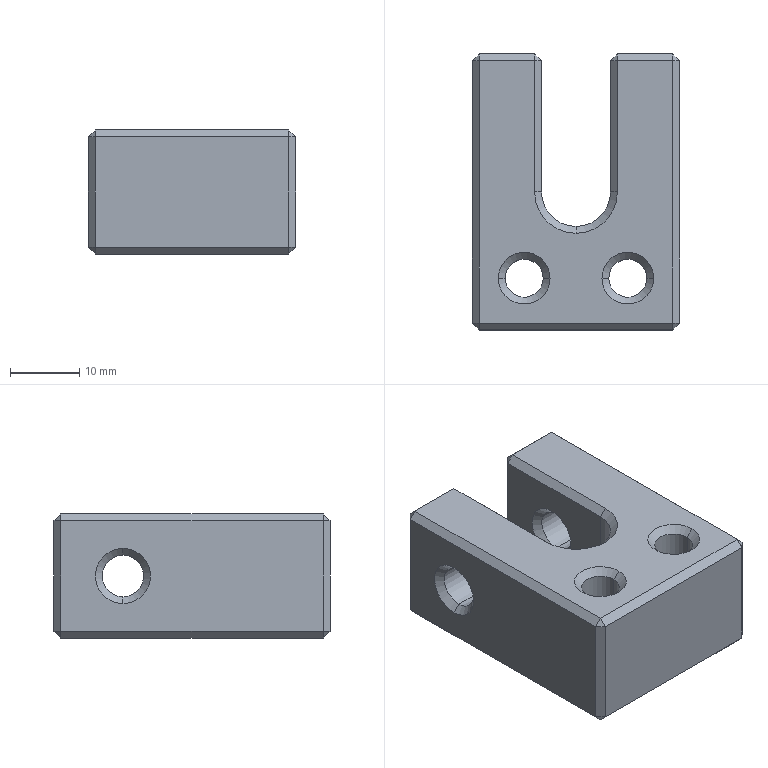Part | STEP file | 1 solid | 75 faces | box 30 x 40 x 18 mm | volume 14417 mm3 | plane 43 | cone 18 | cylinder 14 | commonest cylinder face diameters 5.5 x4 6 x4 9.9 x4 10 x2